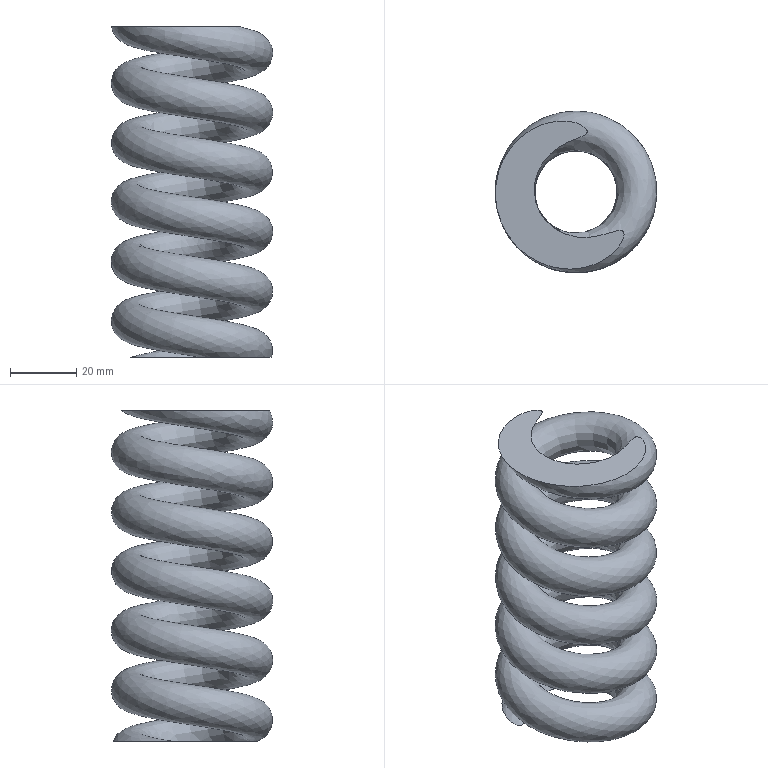Part | NX | features solid 2 | 1 solid | 3 faces | box 48.914 x 48.626 x 100 mm | volume 72503 mm3 | plane 2 | spline 1